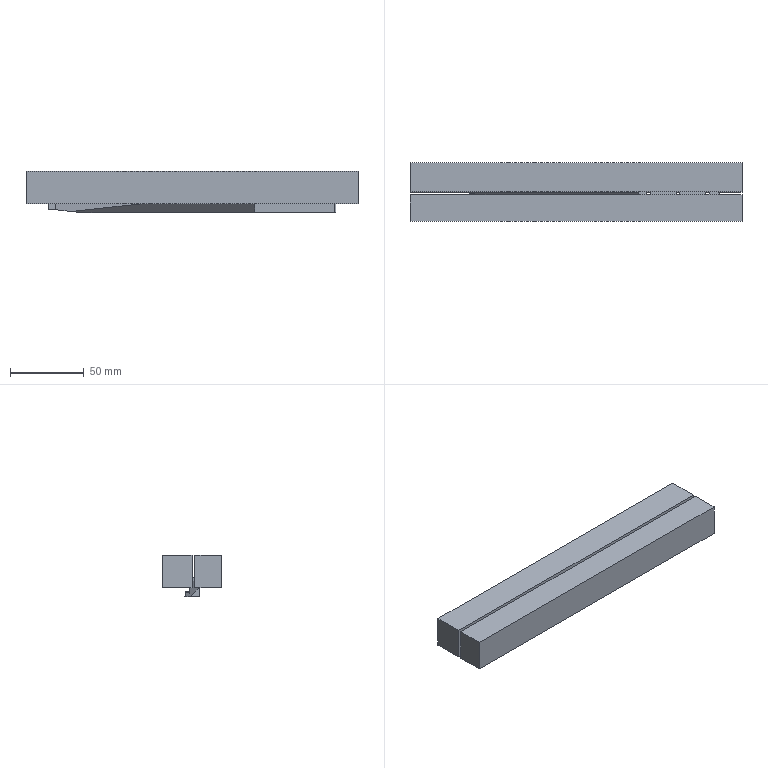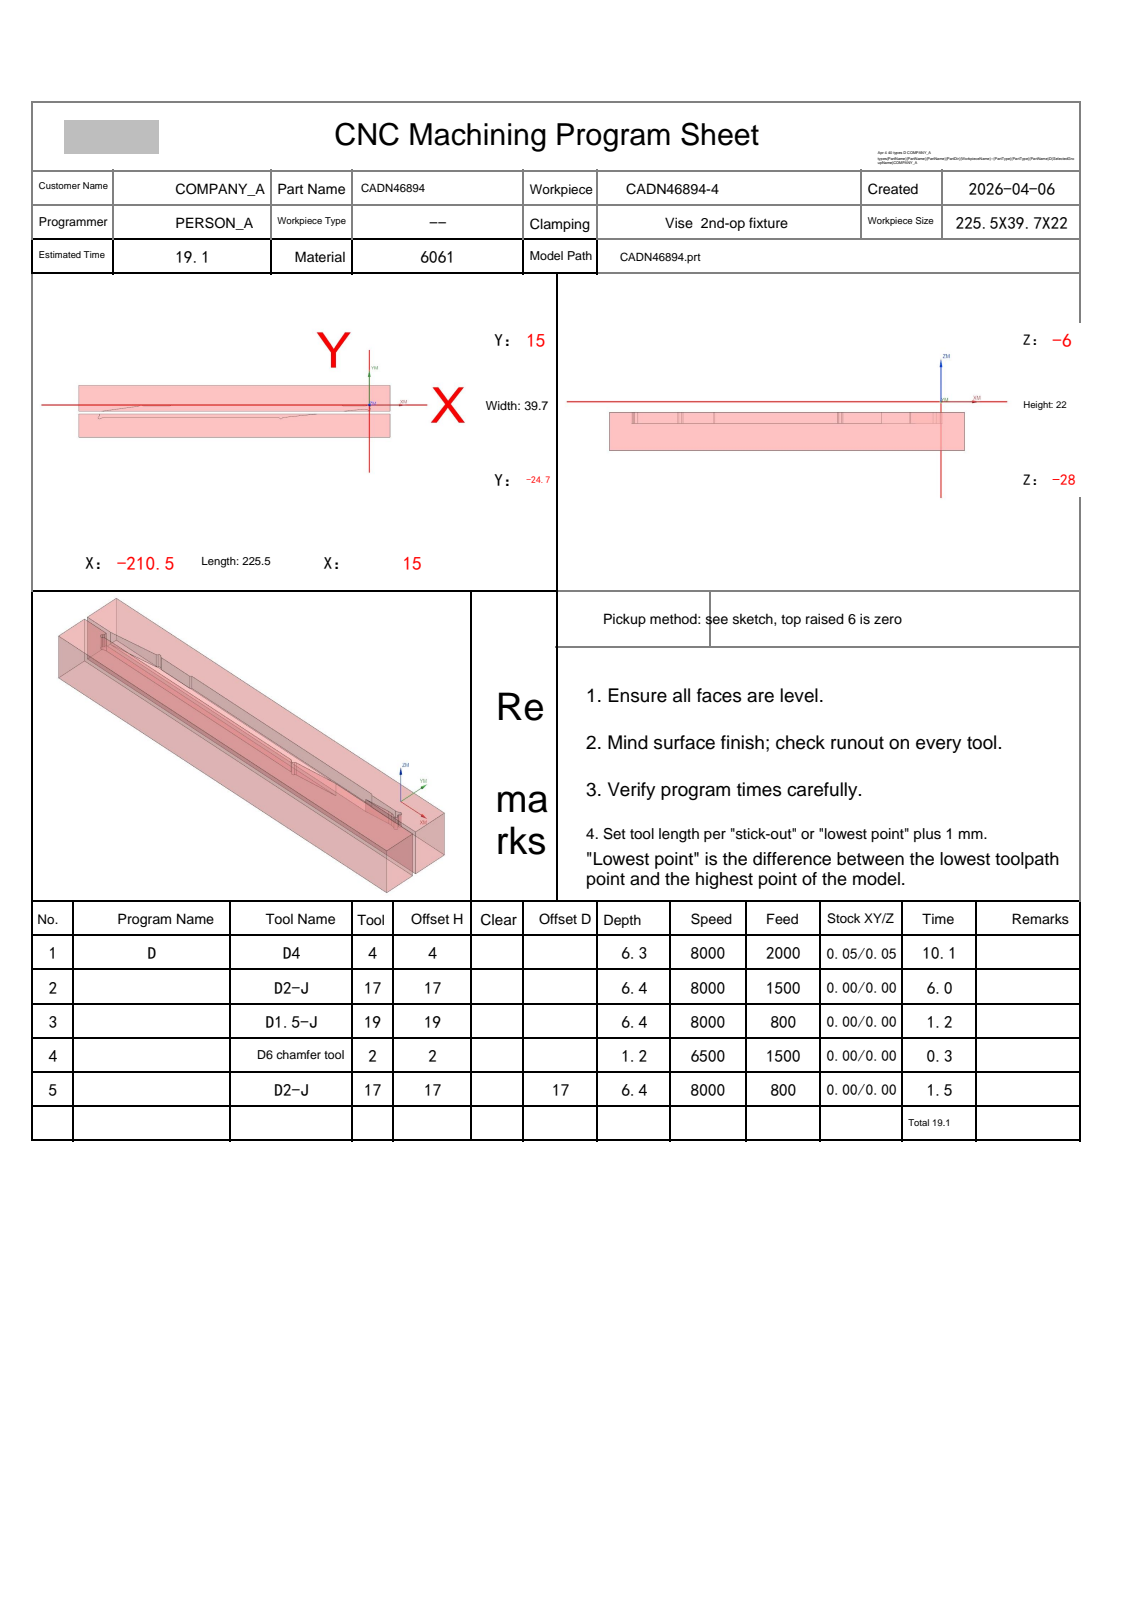NC program | NX | posted by the shop | part box 225.5 x 39.7 x 28 mm
Lines 1401 to 3483 of 3483, first 1748 of 2083 lines:
N8 T17 M06
(D2-J  D=2. R=0. H=17 ce=0.00 di=0.00)
G00 G90 G54 X-41.55 Y4.4 M03 S8000
G43 H17 Z20.
M08
Z-.2
G01 X-41.553 Y4.399 Z-.23 F800.
X-41.56 Y4.397 Z-.258
X-41.571 Y4.394 Z-.282
X-41.585 Y4.389 Z-.304
X-41.602 Y4.383 Z-.323
X-41.62 Y4.375 Z-.34
X-41.64 Y4.365 Z-.354
X-41.66 Y4.353 Z-.366
X-41.68 Y4.339 Z-.376
X-41.698 Y4.322 Z-.384
X-41.715 Y4.303 Z-.39
X-41.729 Y4.282 Z-.395
X-41.74 Y4.257 Z-.398
X-41.747 Y4.23 Z-.399
X-41.75 Y4.2 Z-.4
Y.25
X-37.801
X-37.786 Y.264 Z-.399
X-37.797 Y.305 Z-.396
X-37.831 Y.37 Z-.393
X-37.886 Y.456 Z-.388
X-38.151 Y.812 Z-.373
X-38.406 Y1.125 Z-.364
X-38.606 Y1.361 Z-.362
X-38.843 Y1.63 Z-.363
X-39.12 Y1.936 Z-.369
X-39.43 Y2.266 Z-.38
X-39.756 Y2.602 Z-.394
X-40.077 Y2.923 Z-.41
X-40.375 Y3.211 Z-.426
X-40.639 Y3.457 Z-.441
X-40.872 Y3.665 Z-.453
X-41.185 Y3.93 Z-.47
X-41.541 Y4.207 Z-.489
X-41.629 Y4.265 Z-.494
X-41.694 Y4.301 Z-.497
X-41.736 Y4.313 Z-.499
X-41.75 Y4.3 Z-.5
Y.35
X-37.801
X-37.786 Y.364 Z-.499
X-37.797 Y.405 Z-.496
X-37.831 Y.47 Z-.493
X-37.886 Y.556 Z-.488
X-38.151 Y.912 Z-.473
X-38.406 Y1.225 Z-.464
X-38.606 Y1.461 Z-.462
X-38.843 Y1.73 Z-.463
X-39.12 Y2.036 Z-.469
X-39.43 Y2.366 Z-.48
X-39.756 Y2.702 Z-.494
X-40.077 Y3.023 Z-.51
X-40.375 Y3.311 Z-.526
X-40.639 Y3.557 Z-.541
X-40.872 Y3.765 Z-.553
X-41.185 Y4.03 Z-.57
X-41.541 Y4.307 Z-.589
X-41.629 Y4.365 Z-.594
X-41.694 Y4.401 Z-.597
X-41.736 Y4.413 Z-.599
X-41.75 Y4.4 Z-.6
Y.45
X-37.801
X-37.786 Y.464 Z-.599
X-37.797 Y.504 Z-.596
X-37.831 Y.567 Z-.593
X-37.886 Y.652 Z-.588
X-38.151 Y1.002 Z-.572
X-38.406 Y1.31 Z-.564
X-38.606 Y1.541 Z-.562
X-38.843 Y1.805 Z-.563
X-39.121 Y2.105 Z-.569
X-39.43 Y2.429 Z-.58
X-39.756 Y2.758 Z-.594
X-40.077 Y3.073 Z-.61
X-40.376 Y3.355 Z-.626
X-40.64 Y3.595 Z-.641
X-40.872 Y3.799 Z-.653
X-41.185 Y4.058 Z-.67
X-41.541 Y4.329 Z-.689
X-41.629 Y4.385 Z-.694
X-41.694 Y4.42 Z-.697
X-41.736 Y4.432 Z-.699
X-41.75 Y4.418 Z-.7
Y.55
X-37.81
X-37.795 Y.564 Z-.699
X-37.806 Y.604 Z-.696
X-37.84 Y.669 Z-.693
X-37.895 Y.754 Z-.688
X-38.159 Y1.107 Z-.673
X-38.413 Y1.418 Z-.664
X-38.613 Y1.652 Z-.662
X-38.849 Y1.918 Z-.663
X-39.126 Y2.221 Z-.669
X-39.435 Y2.548 Z-.68
X-39.76 Y2.882 Z-.694
X-40.081 Y3.199 Z-.71
X-40.378 Y3.485 Z-.726
X-40.642 Y3.728 Z-.741
X-40.874 Y3.934 Z-.753
X-41.186 Y4.196 Z-.77
X-41.542 Y4.47 Z-.789
X-41.629 Y4.528 Z-.794
X-41.695 Y4.563 Z-.797
X-41.736 Y4.575 Z-.799
X-41.75 Y4.561 Z-.8
Y.65
X-37.805
X-37.79 Y.664 Z-.799
X-37.801 Y.705 Z-.796
X-37.835 Y.769 Z-.793
X-37.89 Y.856 Z-.788
X-38.155 Y1.21 Z-.773
X-38.409 Y1.524 Z-.764
X-38.609 Y1.759 Z-.762
X-38.846 Y2.027 Z-.763
X-39.123 Y2.332 Z-.769
X-39.432 Y2.661 Z-.78
X-39.758 Y2.997 Z-.794
X-40.079 Y3.317 Z-.81
X-40.377 Y3.604 Z-.826
X-40.64 Y3.849 Z-.841
X-40.873 Y4.057 Z-.853
X-41.185 Y4.321 Z-.87
X-41.542 Y4.597 Z-.889
X-41.629 Y4.655 Z-.894
X-41.695 Y4.691 Z-.897
X-41.736 Y4.703 Z-.899
X-41.75 Y4.69 Z-.9
Y.75
X-37.801
X-37.787 Y.764 Z-.899
X-37.798 Y.805 Z-.896
X-37.832 Y.87 Z-.893
X-37.887 Y.956 Z-.888
X-38.152 Y1.312 Z-.873
X-38.407 Y1.625 Z-.864
X-38.607 Y1.861 Z-.862
X-38.843 Y2.13 Z-.863
X-39.121 Y2.436 Z-.869
X-39.431 Y2.766 Z-.88
X-39.757 Y3.102 Z-.894
X-40.077 Y3.423 Z-.91
X-40.376 Y3.711 Z-.926
X-40.64 Y3.957 Z-.941
X-40.872 Y4.165 Z-.953
X-41.185 Y4.43 Z-.97
X-41.542 Y4.707 Z-.989
X-41.629 Y4.765 Z-.994
X-41.695 Y4.801 Z-.997
X-41.736 Y4.813 Z-.999
X-41.75 Y4.8 Z-1.
Y.85
X-37.8
X-37.786 Y.864 Z-.999
X-37.797 Y.904 Z-.996
X-37.831 Y.968 Z-.993
X-37.886 Y1.054 Z-.988
X-38.151 Y1.406 Z-.973
X-38.406 Y1.716 Z-.964
X-38.606 Y1.949 Z-.962
X-38.843 Y2.215 Z-.963
X-39.121 Y2.517 Z-.969
X-39.43 Y2.843 Z-.98
X-39.756 Y3.176 Z-.994
X-40.077 Y3.492 Z-1.01
X-40.375 Y3.777 Z-1.026
X-40.64 Y4.019 Z-1.041
X-40.872 Y4.225 Z-1.053
X-41.185 Y4.486 Z-1.07
X-41.541 Y4.76 Z-1.089
X-41.629 Y4.817 Z-1.094
X-41.694 Y4.852 Z-1.097
X-41.736 Y4.864 Z-1.099
X-41.75 Y4.85 Z-1.1
Y.948
X-37.801
X-37.787 Y.961 Z-1.099
X-37.798 Y1.001 Z-1.096
X-37.832 Y1.063 Z-1.093
X-37.887 Y1.147 Z-1.088
X-38.152 Y1.491 Z-1.072
X-38.407 Y1.795 Z-1.064
X-38.607 Y2.022 Z-1.062
X-38.844 Y2.282 Z-1.063
X-39.121 Y2.577 Z-1.069
X-39.431 Y2.896 Z-1.08
X-39.757 Y3.221 Z-1.094
X-40.078 Y3.53 Z-1.11
X-40.376 Y3.807 Z-1.126
X-40.64 Y4.044 Z-1.141
X-40.873 Y4.244 Z-1.153
X-41.185 Y4.498 Z-1.17
X-41.542 Y4.764 Z-1.189
X-41.629 Y4.819 Z-1.194
X-41.695 Y4.853 Z-1.197
X-41.736 Y4.864 Z-1.199
X-41.75 Y4.85 Z-1.2
Y1.05
X-37.805
X-37.79 Y1.063 Z-1.199
X-37.801 Y1.102 Z-1.196
X-37.835 Y1.163 Z-1.193
X-37.89 Y1.245 Z-1.188
X-38.155 Y1.581 Z-1.172
X-38.409 Y1.878 Z-1.164
X-38.609 Y2.1 Z-1.162
X-38.846 Y2.353 Z-1.163
X-39.123 Y2.641 Z-1.169
X-39.433 Y2.952 Z-1.18
X-39.759 Y3.268 Z-1.194
X-40.079 Y3.569 Z-1.21
X-40.377 Y3.839 Z-1.226
X-40.641 Y4.069 Z-1.241
X-40.873 Y4.264 Z-1.253
X-41.185 Y4.511 Z-1.27
X-41.542 Y4.768 Z-1.289
X-41.629 Y4.822 Z-1.294
X-41.695 Y4.854 Z-1.297
X-41.736 Y4.864 Z-1.299
X-41.75 Y4.85 Z-1.3
Y1.15
X-37.81
X-37.795 Y1.163 Z-1.299
X-37.806 Y1.201 Z-1.296
X-37.84 Y1.261 Z-1.293
X-37.895 Y1.341 Z-1.288
X-38.159 Y1.669 Z-1.272
X-38.413 Y1.958 Z-1.264
X-38.613 Y2.175 Z-1.262
X-38.849 Y2.423 Z-1.263
X-39.127 Y2.703 Z-1.269
X-39.436 Y3.006 Z-1.28
X-39.761 Y3.314 Z-1.294
X-40.081 Y3.607 Z-1.31
X-40.379 Y3.87 Z-1.326
X-40.642 Y4.094 Z-1.341
X-40.888 Y4.294 Z-1.354
X-41.248 Y4.57 Z-1.374
X-41.542 Y4.773 Z-1.389
X-41.629 Y4.824 Z-1.394
X-41.695 Y4.855 Z-1.397
X-41.736 Y4.865 Z-1.399
X-41.75 Y4.85 Z-1.4
Y1.25
X-37.817
X-37.802 Y1.263 Z-1.399
X-37.813 Y1.299 Z-1.396
X-37.847 Y1.358 Z-1.393
X-37.901 Y1.436 Z-1.388
X-38.166 Y1.757 Z-1.372
X-38.419 Y2.039 Z-1.364
X-38.619 Y2.251 Z-1.362
X-38.854 Y2.492 Z-1.363
X-39.131 Y2.765 Z-1.369
X-39.44 Y3.06 Z-1.38
X-39.765 Y3.36 Z-1.394
X-40.084 Y3.645 Z-1.41
X-40.381 Y3.901 Z-1.426
X-40.644 Y4.118 Z-1.441
X-40.89 Y4.313 Z-1.454
X-41.249 Y4.58 Z-1.474
X-41.542 Y4.777 Z-1.489
X-41.629 Y4.827 Z-1.494
X-41.695 Y4.857 Z-1.497
X-41.736 Y4.865 Z-1.499
X-41.75 Y4.85 Z-1.5
Y1.35
X-37.826
X-37.811 Y1.362 Z-1.499
X-37.822 Y1.398 Z-1.496
X-37.856 Y1.455 Z-1.493
X-37.91 Y1.532 Z-1.488
X-38.125 Y1.79 Z-1.475
X-38.415 Y2.108 Z-1.464
X-38.625 Y2.326 Z-1.462
X-38.861 Y2.561 Z-1.463
X-39.137 Y2.827 Z-1.469
X-39.445 Y3.114 Z-1.48
X-39.769 Y3.406 Z-1.494
X-40.088 Y3.683 Z-1.51
X-40.384 Y3.932 Z-1.526
X-40.647 Y4.143 Z-1.541
X-40.892 Y4.332 Z-1.554
X-41.25 Y4.591 Z-1.574
X-41.543 Y4.782 Z-1.589
X-41.63 Y4.829 Z-1.594
X-41.695 Y4.858 Z-1.597
X-41.736 Y4.865 Z-1.599
X-41.75 Y4.85 Z-1.6
Y1.45
X-37.837
X-37.822 Y1.462 Z-1.599
X-37.833 Y1.497 Z-1.596
X-37.866 Y1.553 Z-1.593
X-37.921 Y1.627 Z-1.588
X-38.135 Y1.879 Z-1.575
X-38.424 Y2.189 Z-1.564
X-38.634 Y2.402 Z-1.562
X-38.869 Y2.63 Z-1.563
X-39.144 Y2.889 Z-1.569
X-39.451 Y3.169 Z-1.58
X-39.774 Y3.452 Z-1.594
X-40.092 Y3.722 Z-1.61
X-40.388 Y3.963 Z-1.626
X-40.653 Y4.171 Z-1.641
X-40.908 Y4.361 Z-1.655
X-41.309 Y4.641 Z-1.677
X-41.543 Y4.786 Z-1.689
X-41.63 Y4.832 Z-1.694
X-41.695 Y4.859 Z-1.697
X-41.736 Y4.866 Z-1.699
X-41.75 Y4.85 Z-1.7
Y1.55
X-37.85
X-37.835 Y1.564 Z-1.699
X-37.851 Y1.605 Z-1.696
X-37.893 Y1.67 Z-1.691
X-37.96 Y1.756 Z-1.686
X-38.217 Y2.044 Z-1.671
X-38.595 Y2.428 Z-1.662
X-38.86 Y2.683 Z-1.663
X-39.142 Y2.942 Z-1.669
X-39.453 Y3.217 Z-1.68
X-39.777 Y3.496 Z-1.694
X-40.096 Y3.759 Z-1.71
X-40.392 Y3.993 Z-1.726
X-40.656 Y4.195 Z-1.741
X-40.911 Y4.38 Z-1.755
X-41.31 Y4.651 Z-1.777
X-41.544 Y4.791 Z-1.789
X-41.63 Y4.835 Z-1.794
X-41.695 Y4.86 Z-1.797
X-41.736 Y4.866 Z-1.799
X-41.75 Y4.85 Z-1.8
Y1.65
X-37.865
X-37.851 Y1.664 Z-1.799
X-37.866 Y1.704 Z-1.796
X-37.908 Y1.767 Z-1.791
X-37.975 Y1.851 Z-1.786
X-38.23 Y2.131 Z-1.771
X-38.607 Y2.505 Z-1.762
X-38.871 Y2.752 Z-1.763
X-39.152 Y3.004 Z-1.769
X-39.461 Y3.272 Z-1.78
X-39.785 Y3.542 Z-1.794
X-40.102 Y3.797 Z-1.81
X-40.397 Y4.024 Z-1.826
X-40.66 Y4.22 Z-1.841
X-40.914 Y4.399 Z-1.855
X-41.312 Y4.66 Z-1.877
X-41.544 Y4.795 Z-1.889
X-41.631 Y4.837 Z-1.894
X-41.695 Y4.861 Z-1.897
X-41.736 Y4.866 Z-1.899
X-41.75 Y4.85 Z-1.9
Y1.75
X-37.882
X-37.868 Y1.764 Z-1.899
X-37.883 Y1.802 Z-1.896
X-37.925 Y1.864 Z-1.891
X-37.991 Y1.946 Z-1.886
X-38.245 Y2.218 Z-1.871
X-38.409 Y2.382 Z-1.865
X-38.622 Y2.587 Z-1.861
X-39.177 Y3.087 Z-1.866
X-39.982 Y3.742 Z-1.903
X-40.655 Y4.237 Z-1.94
X-41.167 Y4.58 Z-1.969
X-41.505 Y4.779 Z-1.987
X-41.607 Y4.829 Z-1.993
X-41.684 Y4.859 Z-1.997
X-41.733 Y4.867 Z-1.999
X-41.75 Y4.85 Z-2.
Y1.85
X-37.902
X-37.887 Y1.863 Z-1.999
X-37.902 Y1.901 Z-1.996
X-37.943 Y1.961 Z-1.991
X-38.009 Y2.04 Z-1.986
X-38.262 Y2.305 Z-1.971
X-38.425 Y2.465 Z-1.965
X-38.682 Y2.705 Z-1.96
X-39.189 Y3.149 Z-1.966
X-39.991 Y3.783 Z-2.003
X-40.676 Y4.272 Z-2.041
X-41.237 Y4.633 Z-2.073
X-41.506 Y4.784 Z-2.087
X-41.608 Y4.833 Z-2.093
X-41.685 Y4.861 Z-2.097
X-41.733 Y4.867 Z-2.099
X-41.75 Y4.85 Z-2.1
Y1.95
X-37.923
X-37.908 Y1.963 Z-2.099
X-37.923 Y2. Z-2.096
X-37.964 Y2.058 Z-2.091
X-38.03 Y2.135 Z-2.086
X-38.281 Y2.392 Z-2.071
X-38.443 Y2.547 Z-2.065
X-38.698 Y2.78 Z-2.06
X-39.202 Y3.211 Z-2.066
X-40. Y3.824 Z-2.103
X-40.681 Y4.297 Z-2.141
X-41.239 Y4.645 Z-2.173
X-41.507 Y4.79 Z-2.187
X-41.609 Y4.836 Z-2.193
X-41.685 Y4.862 Z-2.197
X-41.733 Y4.868 Z-2.199
X-41.75 Y4.85 Z-2.2
Y2.05
X-37.947
X-37.932 Y2.062 Z-2.199
X-37.946 Y2.098 Z-2.196
X-37.987 Y2.155 Z-2.191
X-38.052 Y2.23 Z-2.186
X-38.302 Y2.48 Z-2.171
X-38.462 Y2.629 Z-2.165
X-38.716 Y2.856 Z-2.16
X-39.216 Y3.272 Z-2.166
X-40.009 Y3.866 Z-2.203
X-40.572 Y4.248 Z-2.235
X-40.866 Y4.435 Z-2.252
X-41.242 Y4.656 Z-2.273
X-41.509 Y4.795 Z-2.287
X-41.609 Y4.839 Z-2.293
X-41.685 Y4.864 Z-2.297
X-41.733 Y4.868 Z-2.299
X-41.75 Y4.85 Z-2.3
Y2.15
X-37.972
X-37.958 Y2.162 Z-2.299
X-37.972 Y2.197 Z-2.296
X-38.012 Y2.252 Z-2.291
X-38.076 Y2.324 Z-2.286
X-38.324 Y2.567 Z-2.271
X-38.484 Y2.712 Z-2.265
X-38.735 Y2.931 Z-2.26
X-39.232 Y3.334 Z-2.266
X-40.02 Y3.907 Z-2.303
X-40.58 Y4.276 Z-2.335
X-40.872 Y4.455 Z-2.352
X-41.245 Y4.667 Z-2.373
X-41.51 Y4.8 Z-2.387
X-41.61 Y4.842 Z-2.393
X-41.686 Y4.865 Z-2.397
X-41.733 Y4.868 Z-2.399
X-41.75 Y4.85 Z-2.4
Y2.25
X-38.
X-37.986 Y2.262 Z-2.399
X-37.999 Y2.295 Z-2.396
X-38.039 Y2.348 Z-2.391
X-38.103 Y2.419 Z-2.386
X-38.297 Y2.607 Z-2.374
X-38.513 Y2.8 Z-2.365
X-38.8 Y3.042 Z-2.36
X-39.25 Y3.396 Z-2.366
X-40.032 Y3.948 Z-2.403
X-40.587 Y4.303 Z-2.435
X-40.877 Y4.476 Z-2.452
X-41.248 Y4.679 Z-2.473
X-41.512 Y4.806 Z-2.487
X-41.611 Y4.845 Z-2.493
X-41.686 Y4.867 Z-2.497
X-41.733 Y4.869 Z-2.499
X-41.75 Y4.85 Z-2.5
Y2.35
X-38.031
X-38.016 Y2.361 Z-2.499
X-38.029 Y2.394 Z-2.496
X-38.069 Y2.445 Z-2.491
X-38.132 Y2.514 Z-2.486
X-38.324 Y2.696 Z-2.474
X-38.538 Y2.882 Z-2.465
X-38.823 Y3.117 Z-2.46
X-39.268 Y3.457 Z-2.466
X-39.922 Y3.91 Z-2.496
X-40.574 Y4.317 Z-2.533
X-40.896 Y4.502 Z-2.552
X-41.316 Y4.722 Z-2.576
X-41.513 Y4.811 Z-2.587
X-41.612 Y4.848 Z-2.593
X-41.687 Y4.868 Z-2.597
X-41.734 Y4.869 Z-2.599
X-41.75 Y4.85 Z-2.6
Y2.45
X-38.063
X-38.048 Y2.461 Z-2.599
X-38.061 Y2.492 Z-2.596
X-38.1 Y2.542 Z-2.591
X-38.162 Y2.608 Z-2.586
X-38.353 Y2.784 Z-2.574
X-38.565 Y2.965 Z-2.565
X-38.847 Y3.191 Z-2.56
X-39.288 Y3.519 Z-2.566
X-39.716 Y3.813 Z-2.584
X-40.158 Y4.096 Z-2.608
X-40.756 Y4.444 Z-2.644
X-41.028 Y4.588 Z-2.66
X-41.396 Y4.767 Z-2.681
X-41.515 Y4.816 Z-2.687
X-41.613 Y4.851 Z-2.693
X-41.687 Y4.869 Z-2.697
X-41.734 Y4.87 Z-2.699
X-41.75 Y4.85 Z-2.7
Y2.55
X-38.098
X-38.083 Y2.561 Z-2.699
X-38.096 Y2.591 Z-2.696
X-38.134 Y2.639 Z-2.691
X-38.196 Y2.703 Z-2.686
X-38.384 Y2.873 Z-2.674
X-38.594 Y3.047 Z-2.665
X-38.873 Y3.265 Z-2.66
X-39.31 Y3.581 Z-2.666
X-39.734 Y3.863 Z-2.684
X-40.171 Y4.134 Z-2.708
X-40.764 Y4.467 Z-2.744
X-41.034 Y4.605 Z-2.76
X-41.399 Y4.775 Z-2.781
X-41.517 Y4.822 Z-2.787
X-41.614 Y4.854 Z-2.793
X-41.687 Y4.871 Z-2.797
X-41.734 Y4.87 Z-2.799
X-41.75 Y4.85 Z-2.8
Y2.65
X-38.136
X-38.12 Y2.66 Z-2.799
X-38.133 Y2.69 Z-2.796
X-38.17 Y2.736 Z-2.791
X-38.231 Y2.798 Z-2.786
X-38.417 Y2.961 Z-2.774
X-38.625 Y3.129 Z-2.765
X-38.9 Y3.339 Z-2.76
X-39.333 Y3.642 Z-2.766
X-39.752 Y3.913 Z-2.784
X-40.186 Y4.173 Z-2.808
X-40.773 Y4.491 Z-2.844
X-41.04 Y4.622 Z-2.86
X-41.402 Y4.783 Z-2.881
X-41.519 Y4.827 Z-2.887
X-41.615 Y4.857 Z-2.893
X-41.688 Y4.872 Z-2.897
X-41.734 Y4.87 Z-2.899
X-41.75 Y4.85 Z-2.9
Y2.75
X-38.176
X-38.16 Y2.76 Z-2.899
X-38.172 Y2.788 Z-2.896
X-38.209 Y2.833 Z-2.891
X-38.269 Y2.892 Z-2.886
X-38.405 Y3.011 Z-2.876
X-38.647 Y3.204 Z-2.865
X-38.93 Y3.413 Z-2.86
X-39.358 Y3.704 Z-2.866
X-39.772 Y3.963 Z-2.884
X-40.201 Y4.211 Z-2.908
X-40.783 Y4.514 Z-2.944
X-41.047 Y4.639 Z-2.96
X-41.405 Y4.791 Z-2.981
X-41.521 Y4.832 Z-2.987
X-41.616 Y4.86 Z-2.993
X-41.689 Y4.874 Z-2.997
X-41.734 Y4.871 Z-2.999
X-41.75 Y4.85 Z-3.
Y2.85
X-38.218
X-38.202 Y2.862 Z-2.999
X-38.22 Y2.895 Z-2.995
X-38.267 Y2.947 Z-2.989
X-38.341 Y3.016 Z-2.983
X-38.562 Y3.195 Z-2.97
X-38.721 Y3.315 Z-2.964
X-39. Y3.514 Z-2.959
X-39.384 Y3.766 Z-2.966
X-39.793 Y4.013 Z-2.984
X-40.217 Y4.25 Z-3.008
X-40.793 Y4.537 Z-3.044
X-41.054 Y4.656 Z-3.06
X-41.409 Y4.799 Z-3.081
X-41.523 Y4.838 Z-3.087
X-41.618 Y4.863 Z-3.093
X-41.689 Y4.875 Z-3.097
X-41.734 Y4.871 Z-3.099
X-41.75 Y4.85 Z-3.1
Y2.95
X-38.263
X-38.247 Y2.961 Z-3.099
X-38.264 Y2.993 Z-3.095
X-38.31 Y3.044 Z-3.089
X-38.383 Y3.11 Z-3.083
X-38.601 Y3.282 Z-3.07
X-38.757 Y3.396 Z-3.064
X-39.032 Y3.587 Z-3.059
X-39.411 Y3.827 Z-3.066
X-39.816 Y4.063 Z-3.084
X-40.234 Y4.288 Z-3.108
X-40.803 Y4.561 Z-3.144
X-41.062 Y4.672 Z-3.16
X-41.412 Y4.808 Z-3.181
X-41.526 Y4.843 Z-3.187
X-41.619 Y4.867 Z-3.193
X-41.69 Y4.876 Z-3.197
X-41.734 Y4.871 Z-3.199
X-41.75 Y4.85 Z-3.2
Y3.05
X-38.311
X-38.294 Y3.061 Z-3.199
X-38.311 Y3.092 Z-3.195
X-38.356 Y3.14 Z-3.189
X-38.428 Y3.203 Z-3.183
X-38.588 Y3.328 Z-3.173
X-38.796 Y3.478 Z-3.164
X-39.067 Y3.659 Z-3.159
X-39.441 Y3.889 Z-3.166
X-39.84 Y4.113 Z-3.184
X-40.253 Y4.326 Z-3.208
X-40.777 Y4.569 Z-3.241
X-41.024 Y4.671 Z-3.257
X-41.346 Y4.793 Z-3.276
X-41.481 Y4.835 Z-3.284
X-41.592 Y4.864 Z-3.291
X-41.677 Y4.877 Z-3.296
X-41.731 Y4.873 Z-3.299
X-41.75 Y4.85 Z-3.3
Y3.15
X-38.361
X-38.345 Y3.16 Z-3.299
X-38.36 Y3.19 Z-3.295
X-38.405 Y3.236 Z-3.289
X-38.475 Y3.297 Z-3.283
X-38.632 Y3.416 Z-3.273
X-38.837 Y3.559 Z-3.264
X-39.104 Y3.732 Z-3.259
X-39.472 Y3.95 Z-3.266
X-39.865 Y4.163 Z-3.284
X-40.272 Y4.365 Z-3.308
X-40.79 Y4.593 Z-3.341
X-41.033 Y4.689 Z-3.357
X-41.351 Y4.803 Z-3.376
X-41.484 Y4.842 Z-3.384
X-41.594 Y4.868 Z-3.391
X-41.678 Y4.879 Z-3.396
X-41.731 Y4.874 Z-3.399
X-41.75 Y4.85 Z-3.4
Y3.25
X-38.414
X-38.398 Y3.26 Z-3.399
X-38.413 Y3.288 Z-3.395
X-38.456 Y3.332 Z-3.389
X-38.525 Y3.39 Z-3.383
X-38.679 Y3.504 Z-3.373
X-38.88 Y3.64 Z-3.364
X-39.143 Y3.805 Z-3.359
X-39.505 Y4.012 Z-3.366
X-39.891 Y4.213 Z-3.384
X-40.292 Y4.403 Z-3.408
X-40.803 Y4.617 Z-3.441
X-41.043 Y4.707 Z-3.457
X-41.357 Y4.812 Z-3.476
X-41.487 Y4.848 Z-3.484
X-41.596 Y4.872 Z-3.491
X-41.679 Y4.881 Z-3.496
X-41.732 Y4.874 Z-3.499
X-41.75 Y4.85 Z-3.5
Y3.35
X-38.47
X-38.454 Y3.359 Z-3.499
X-38.468 Y3.386 Z-3.495
X-38.51 Y3.429 Z-3.489
X-38.577 Y3.484 Z-3.483
X-38.667 Y3.55 Z-3.476
X-38.913 Y3.713 Z-3.465
X-39.184 Y3.878 Z-3.459
X-39.539 Y4.074 Z-3.466
X-39.92 Y4.263 Z-3.484
X-40.314 Y4.441 Z-3.508
X-40.816 Y4.641 Z-3.541
X-41.053 Y4.725 Z-3.557
X-41.362 Y4.822 Z-3.576
X-41.491 Y4.855 Z-3.584
X-41.598 Y4.875 Z-3.591
X-41.68 Y4.882 Z-3.596
X-41.732 Y4.875 Z-3.599
X-41.75 Y4.85 Z-3.6
Y3.45
X-38.53
X-38.513 Y3.459 Z-3.599
X-38.526 Y3.485 Z-3.595
X-38.567 Y3.525 Z-3.589
X-38.633 Y3.577 Z-3.583
X-38.72 Y3.64 Z-3.576
X-38.961 Y3.795 Z-3.565
X-39.227 Y3.951 Z-3.559
X-39.576 Y4.135 Z-3.566
X-39.949 Y4.313 Z-3.584
X-40.337 Y4.48 Z-3.608
X-40.831 Y4.666 Z-3.641
X-41.064 Y4.743 Z-3.657
X-41.368 Y4.832 Z-3.676
X-41.495 Y4.861 Z-3.684
X-41.6 Y4.879 Z-3.691
X-41.681 Y4.884 Z-3.696
X-41.732 Y4.875 Z-3.699
X-41.75 Y4.85 Z-3.7
Y3.55
X-38.592
X-38.575 Y3.559 Z-3.699
X-38.588 Y3.583 Z-3.695
X-38.627 Y3.621 Z-3.689
X-38.691 Y3.671 Z-3.683
X-38.777 Y3.73 Z-3.676
X-39.012 Y3.877 Z-3.665
X-39.272 Y4.024 Z-3.659
X-39.614 Y4.197 Z-3.666
X-39.98 Y4.363 Z-3.684
X-40.361 Y4.518 Z-3.708
X-40.846 Y4.69 Z-3.742
X-41.075 Y4.761 Z-3.757
X-41.374 Y4.842 Z-3.776
X-41.499 Y4.868 Z-3.784
X-41.603 Y4.883 Z-3.791
X-41.682 Y4.886 Z-3.796
X-41.732 Y4.875 Z-3.799
X-41.75 Y4.85 Z-3.8
Y3.65
X-38.658
X-38.64 Y3.658 Z-3.799
X-38.652 Y3.681 Z-3.795
X-38.691 Y3.717 Z-3.789
X-38.753 Y3.764 Z-3.783
X-38.836 Y3.82 Z-3.776
X-39.066 Y3.959 Z-3.765
X-39.32 Y4.097 Z-3.759
X-39.655 Y4.259 Z-3.766
X-40.013 Y4.413 Z-3.784
X-40.386 Y4.556 Z-3.808
X-40.862 Y4.714 Z-3.842
X-41.087 Y4.779 Z-3.857
X-41.38 Y4.851 Z-3.876
X-41.503 Y4.874 Z-3.884
X-41.605 Y4.887 Z-3.891
X-41.683 Y4.888 Z-3.896
X-41.733 Y4.876 Z-3.899
X-41.75 Y4.85 Z-3.9
Y3.75
X-38.727
X-38.709 Y3.76 Z-3.898
X-38.727 Y3.787 Z-3.894
X-38.777 Y3.829 Z-3.887
X-38.856 Y3.883 Z-3.88
X-38.958 Y3.947 Z-3.872
X-39.157 Y4.059 Z-3.863
X-39.371 Y4.17 Z-3.859
X-39.698 Y4.32 Z-3.866
X-40.048 Y4.463 Z-3.884
X-40.412 Y4.595 Z-3.908
X-40.83 Y4.725 Z-3.938
X-41.099 Y4.797 Z-3.957
X-41.387 Y4.861 Z-3.976
X-41.508 Y4.881 Z-3.984
X-41.608 Y4.89 Z-3.991
X-41.684 Y4.889 Z-3.996
X-41.733 Y4.876 Z-3.999
X-41.75 Y4.85 Z-4.
Y3.85
X-38.801
X-38.782 Y3.859 Z-3.998
X-38.799 Y3.885 Z-3.994
X-38.847 Y3.924 Z-3.987
X-38.923 Y3.975 Z-3.98
X-39.023 Y4.035 Z-3.972
X-39.216 Y4.14 Z-3.963
X-39.424 Y4.243 Z-3.959
X-39.743 Y4.382 Z-3.966
X-40.085 Y4.513 Z-3.984
X-40.44 Y4.633 Z-4.008
X-40.848 Y4.751 Z-4.038
X-41.112 Y4.815 Z-4.057
X-41.394 Y4.871 Z-4.076
X-41.512 Y4.887 Z-4.084
X-41.611 Y4.894 Z-4.091
X-41.686 Y4.891 Z-4.096
X-41.733 Y4.877 Z-4.099
X-41.75 Y4.85 Z-4.1
Y3.95
X-38.877
X-38.859 Y3.959 Z-4.098
X-38.874 Y3.983 Z-4.094
X-38.92 Y4.02 Z-4.087
X-38.994 Y4.067 Z-4.08
X-39.09 Y4.123 Z-4.072
X-39.278 Y4.22 Z-4.063
X-39.48 Y4.316 Z-4.059
X-39.79 Y4.444 Z-4.066
X-40.123 Y4.563 Z-4.084
X-40.47 Y4.671 Z-4.108
X-40.868 Y4.776 Z-4.138
X-41.126 Y4.833 Z-4.157
X-41.402 Y4.881 Z-4.176
X-41.517 Y4.894 Z-4.184
X-41.614 Y4.898 Z-4.191
X-41.687 Y4.893 Z-4.196
X-41.734 Y4.877 Z-4.199
X-41.75 Y4.85 Z-4.2
Y4.05
X-38.959
X-38.939 Y4.058 Z-4.198
X-38.953 Y4.08 Z-4.194
X-38.998 Y4.115 Z-4.187
X-39.068 Y4.159 Z-4.18
X-39.162 Y4.211 Z-4.172
X-39.274 Y4.268 Z-4.166
X-39.401 Y4.328 Z-4.161
X-39.54 Y4.389 Z-4.159
X-39.84 Y4.505 Z-4.166
X-40.164 Y4.613 Z-4.184
X-40.501 Y4.71 Z-4.208
X-40.899 Y4.804 Z-4.239
X-41.092 Y4.842 Z-4.253
X-41.332 Y4.881 Z-4.271
X-41.468 Y4.896 Z-4.281
X-41.584 Y4.902 Z-4.289
X-41.673 Y4.897 Z-4.295
X-41.73 Y4.88 Z-4.299
X-41.75 Y4.85 Z-4.3
Y4.15
X-39.044
X-39.024 Y4.157 Z-4.298
X-39.037 Y4.178 Z-4.294
X-39.079 Y4.21 Z-4.287
X-39.147 Y4.251 Z-4.28
X-39.237 Y4.299 Z-4.272
X-39.345 Y4.351 Z-4.266
X-39.468 Y4.406 Z-4.261
X-39.602 Y4.462 Z-4.259
X-39.893 Y4.567 Z-4.266
X-40.206 Y4.663 Z-4.284
X-40.534 Y4.748 Z-4.308
X-40.92 Y4.829 Z-4.339
X-41.108 Y4.861 Z-4.353
X-41.342 Y4.893 Z-4.371
X-41.475 Y4.904 Z-4.381
X-41.588 Y4.907 Z-4.389
X-41.675 Y4.899 Z-4.395
X-41.73 Y4.881 Z-4.399
X-41.75 Y4.85 Z-4.4
Y4.25
X-39.134
X-39.114 Y4.257 Z-4.398
X-39.125 Y4.276 Z-4.394
X-39.165 Y4.305 Z-4.387
X-39.23 Y4.343 Z-4.38
X-39.316 Y4.387 Z-4.372
X-39.42 Y4.435 Z-4.366
X-39.538 Y4.484 Z-4.361
X-39.668 Y4.534 Z-4.359
X-39.949 Y4.629 Z-4.366
X-40.252 Y4.713 Z-4.384
X-40.569 Y4.786 Z-4.408
X-40.943 Y4.855 Z-4.439
X-41.126 Y4.881 Z-4.453
X-41.353 Y4.905 Z-4.471
X-41.483 Y4.912 Z-4.481
X-41.592 Z-4.489
X-41.677 Y4.902 Z-4.495
X-41.731 Y4.881 Z-4.499
X-41.75 Y4.85 Z-4.5
Y4.35
X-39.23
X-39.209 Y4.356 Z-4.498
X-39.219 Y4.374 Z-4.494
X-39.256 Y4.401 Z-4.487
X-39.318 Y4.435 Z-4.48
X-39.4 Y4.475 Z-4.472
X-39.499 Y4.518 Z-4.466
X-39.613 Y4.563 Z-4.461
X-39.737 Y4.607 Z-4.459
X-40.008 Y4.69 Z-4.466
X-40.299 Y4.763 Z-4.484
X-40.605 Y4.825 Z-4.508
X-40.968 Y4.88 Z-4.539
X-41.144 Y4.9 Z-4.553
X-41.364 Y4.917 Z-4.571
X-41.49 Y4.921 Z-4.581
X-41.597 Y4.916 Z-4.589
X-41.679 Y4.904 Z-4.595
X-41.731 Y4.882 Z-4.599
X-41.75 Y4.85 Z-4.6
Y4.45
X-39.331
X-39.309 Y4.456 Z-4.598
X-39.317 Y4.472 Z-4.594
X-39.352 Y4.496 Z-4.587
X-39.41 Y4.527 Z-4.58
X-39.488 Y4.562 Z-4.572
X-39.583 Y4.601 Z-4.566
X-39.692 Y4.641 Z-4.561
X-39.811 Y4.68 Z-4.559
X-40.07 Y4.752 Z-4.566
X-40.35 Y4.813 Z-4.584
X-40.644 Y4.863 Z-4.608
X-40.994 Y4.905 Z-4.639
X-41.164 Y4.919 Z-4.653
X-41.377 Y4.929 Z-4.671
X-41.498 Z-4.681
X-41.601 Y4.921 Z-4.689
X-41.681 Y4.906 Z-4.695
X-41.732 Y4.883 Z-4.699
X-41.75 Y4.85 Z-4.7
Y4.55
X-39.437
X-39.415 Y4.557 Z-4.698
X-39.429 Y4.575 Z-4.692
X-39.475 Y4.602 Z-4.684
X-39.549 Y4.636 Z-4.675
X-39.645 Y4.675 Z-4.667
X-39.76 Y4.714 Z-4.662
X-39.889 Y4.753 Z-4.659
X-40.136 Y4.814 Z-4.666
X-40.403 Y4.863 Z-4.684
X-40.685 Y4.901 Z-4.708
X-41.021 Y4.931 Z-4.739
X-41.185 Y4.939 Z-4.753
X-41.389 Y4.942 Z-4.771
X-41.507 Y4.937 Z-4.781
X-41.606 Y4.926 Z-4.789
X-41.683 Y4.908 Z-4.795
X-41.733 Y4.883 Z-4.799
X-41.75 Y4.85 Z-4.8
Y4.65
X-39.551
X-39.549 Y4.653 Z-4.799
X-39.582 Y4.66 Z-4.795
X-39.825 Y4.697 Z-4.782
X-40.115 Y4.73 Z-4.774
X-40.469 Y4.757 Z-4.777
X-40.837 Y4.773 Z-4.793
X-41.191 Y4.776 Z-4.82
X-41.481 Y4.768 Z-4.853
X-41.724 Y4.755 Z-4.89
X-41.757 Y4.751 Z-4.897
X-41.755 Y4.75 Z-4.9
X-39.672
X-39.668 Y4.753 Z-4.899
X-39.699 Y4.76 Z-4.895
X-39.928 Y4.797 Z-4.882
X-40.201 Y4.83 Z-4.874
X-40.536 Y4.857 Z-4.877
X-40.885 Y4.873 Z-4.893
X-41.22 Y4.876 Z-4.92
X-41.494 Y4.868 Z-4.953
X-41.723 Y4.855 Z-4.99
X-41.753 Y4.851 Z-4.997
X-41.75 Y4.85 Z-5.
X-39.801
X-39.796 Y4.853 Z-4.999
X-39.824 Y4.86 Z-4.995
X-39.973 Y4.887 Z-4.985
X-40.086 Y4.904 Z-4.98
X-40.297 Y4.93 Z-4.974
X-40.613 Y4.957 Z-4.977
X-40.942 Y4.973 Z-4.993
X-41.259 Y4.976 Z-5.02
X-41.469 Y4.97 Z-5.046
X-41.583 Y4.965 Z-5.063
X-41.731 Y4.955 Z-5.09
X-41.759 Y4.951 Z-5.097
X-41.755 Y4.95 Z-5.1
X-39.939
X-39.933 Y4.952 Z-5.099
X-39.95 Y4.958 Z-5.096
X-39.988 Y4.967 Z-5.093
X-40.18 Y5. Z-5.081
X-40.401 Y5.03 Z-5.074
X-40.699 Y5.057 Z-5.077
X-41.01 Y5.073 Z-5.093
X-41.308 Y5.076 Z-5.12
X-41.528 Y5.069 Z-5.15
X-41.721 Y5.057 Z-5.183
X-41.759 Y5.054 Z-5.192
X-41.776 Y5.051 Z-5.198
X-41.77 Y5.05 Z-5.2
X-40.088
X-40.081 Y5.052 Z-5.199
X-40.096 Y5.058 Z-5.196
X-40.131 Y5.067 Z-5.193
X-40.258 Y5.092 Z-5.183
X-40.351 Y5.107 Z-5.179
X-40.517 Y5.13 Z-5.174
X-40.724 Y5.151 Z-5.175
X-40.942 Y5.166 Z-5.184
X-41.159 Y5.175 Z-5.199
X-41.367 Y5.176 Z-5.22
X-41.533 Y5.171 Z-5.243
X-41.625 Y5.167 Z-5.258
X-41.752 Y5.157 Z-5.283
X-41.787 Y5.154 Z-5.292
X-41.803 Y5.151 Z-5.298
X-41.796 Y5.15 Z-5.3
X-40.249
X-40.242 Y5.152 Z-5.299
X-40.255 Y5.158 Z-5.296
X-40.287 Y5.167 Z-5.293
X-40.404 Y5.192 Z-5.283
X-40.49 Y5.207 Z-5.279
X-40.645 Y5.23 Z-5.274
X-40.838 Y5.251 Z-5.275
X-41.041 Y5.266 Z-5.284
X-41.244 Y5.275 Z-5.299
X-41.438 Y5.276 Z-5.32
X-41.592 Y5.271 Z-5.343
X-41.678 Y5.267 Z-5.358
X-41.796 Y5.257 Z-5.383
X-41.828 Y5.254 Z-5.392
X-41.841 Y5.251 Z-5.398
X-41.833 Y5.25 Z-5.4
X-40.426
X-40.417 Y5.252 Z-5.399
X-40.429 Y5.258 Z-5.396
X-40.458 Y5.267 Z-5.393
X-40.502 Y5.278 Z-5.388
X-40.637 Y5.305 Z-5.379
X-40.787 Y5.33 Z-5.374
X-40.967 Y5.351 Z-5.375
X-41.155 Y5.366 Z-5.384
X-41.343 Y5.375 Z-5.399
X-41.522 Y5.376 Z-5.42
X-41.673 Y5.371 Z-5.445
X-41.808 Y5.362 Z-5.472
X-41.852 Y5.357 Z-5.483
X-41.881 Y5.354 Z-5.492
X-41.892 Y5.351 Z-5.498
X-41.884 Y5.35 Z-5.5
X-40.621
X-40.612 Y5.352 Z-5.499
X-40.621 Y5.358 Z-5.496
X-40.647 Y5.367 Z-5.493
X-40.687 Y5.378 Z-5.488
X-40.774 Y5.398 Z-5.481
X-40.839 Y5.411 Z-5.478
X-40.948 Y5.43 Z-5.474
X-41.112 Y5.451 Z-5.475
X-41.286 Y5.466 Z-5.484
X-41.459 Y5.475 Z-5.499
X-41.623 Y5.476 Z-5.52
X-41.732 Y5.472 Z-5.539
X-41.797 Y5.469 Z-5.552
X-41.884 Y5.462 Z-5.572
X-41.924 Y5.457 Z-5.583
X-41.95 Y5.454 Z-5.592
X-41.959 Y5.451 Z-5.598
X-41.95 Y5.45 Z-5.6
X-40.841
X-40.831 Y5.452 Z-5.599
X-40.838 Y5.458 Z-5.596
X-40.86 Y5.467 Z-5.593
X-40.896 Y5.478 Z-5.588
X-40.942 Y5.491 Z-5.584
X-40.998 Y5.504 Z-5.579
X-41.062 Y5.517 Z-5.576
X-41.131 Y5.53 Z-5.574
X-41.281 Y5.551 Z-5.575
X-41.438 Y5.566 Z-5.584
X-41.596 Y5.575 Z-5.599
X-41.746 Y5.576 Z-5.62
X-41.815 Y5.574 Z-5.633
X-41.878 Y5.571 Z-5.646
X-41.935 Y5.566 Z-5.659
X-41.981 Y5.562 Z-5.672
X-42.016 Y5.557 Z-5.683
X-42.038 Y5.554 Z-5.692
X-42.046 Y5.551 Z-5.698
X-42.036 Y5.55 Z-5.7
X-41.095
X-41.084 Y5.552 Z-5.699
X-41.089 Y5.558 Z-5.696
X-41.108 Y5.567 Z-5.693
X-41.138 Y5.578 Z-5.688
X-41.179 Y5.591 Z-5.684
X-41.229 Y5.604 Z-5.679
X-41.285 Y5.617 Z-5.676
X-41.347 Y5.63 Z-5.674
X-41.481 Y5.651 Z-5.675
X-41.622 Y5.666 Z-5.684
X-41.764 Y5.675 Z-5.699
X-41.898 Y5.676 Z-5.72
X-41.959 Y5.674 Z-5.733
X-42.016 Y5.671 Z-5.746
X-42.066 Y5.666 Z-5.759
X-42.106 Y5.662 Z-5.772
X-42.137 Y5.657 Z-5.783
X-42.156 Y5.654 Z-5.792
X-42.161 Y5.651 Z-5.798
X-42.15 Y5.65 Z-5.8
X-41.401
X-41.375 Y5.653 Z-5.798
X-41.364 Y5.661 Z-5.792
X-41.366 Y5.673 Z-5.784
X-41.38 Y5.689 Z-5.774
X-41.404 Y5.707 Z-5.763
X-41.438 Y5.726 Z-5.751
X-41.48 Y5.746 Z-5.739
X-41.528 Y5.765 Z-5.729
X-41.581 Y5.783 Z-5.721
X-41.687 Y5.809 Z-5.713
X-41.8 Y5.827 Z-5.714
X-41.915 Y5.836 Z-5.723
X-42.028 Y5.837 Z-5.741
X-42.133 Y5.829 Z-5.767
X-42.187 Y5.821 Z-5.785
X-42.235 Y5.811 Z-5.804
X-42.276 Y5.799 Z-5.824
X-42.31 Y5.787 Z-5.843
X-42.335 Y5.776 Z-5.861
X-42.349 Y5.766 Z-5.877
X-42.351 Y5.758 Z-5.889
X-42.34 Y5.752 Z-5.897
X-42.314 Y5.75 Z-5.9
X-41.806
X-41.773 Y5.752 Z-5.897
X-41.744 Y5.758 Z-5.889
X-41.718 Y5.767 Z-5.877
X-41.696 Y5.778 Z-5.86
X-41.676 Y5.791 Z-5.84
X-41.66 Y5.806 Z-5.816
X-41.646 Y5.821 Z-5.789
X-41.634 Y5.836 Z-5.76
X-41.624 Y5.85 Z-5.729
X-41.617 Y5.863 Z-5.696
X-41.612 Y5.875 Z-5.662
X-41.608 Y5.884 Z-5.628
X-41.606 Y5.889 Z-5.593
Y5.891 Z-5.559
G00 Z20.
G91 G28 Z0.0
M05
M09
G91 G28 Z0.0
M01
N9 T18 M06
(D4R0.5  D=4. R=0.5 H=18 ce=0.00 di=0.00)
G00 G90 G54 X78.892 Y-4.82 M03 S6000
G43 H18 Z20.
M08
Z2.989
G01 Z-.103 F3500.
X76.902 Y-4.627 Z-.025
X76.067 Y-4.547 Z.007
X75.798 Y-4.521 Z.015
Y-4.421
X76.067 Y-4.447 Z.008
X77.995 Y-4.633 Z-.068
X79.087 Y-4.639 Z-.111
X76.067 Y-4.347 Z.008
X75.798 Y-4.321 Z.015
Y-4.221
X76.067 Y-4.247 Z.008
X80.165 Y-4.643 Z-.153
X81.229 Y-4.645 Z-.195
X76.067 Y-4.147 Z.008
X75.798 Y-4.121 Z.015
Y-4.021
X76.067 Y-4.047 Z.008
X82.286 Y-4.648 Z-.236
X83.327 Z-.277
X76.067 Y-3.947 Z.008
X75.798 Y-3.921 Z.015
Y-3.821
X76.067 Y-3.847 Z.008
X84.367 Y-4.649 Z-.317
X85.407 Z-.358
X76.067 Y-3.747 Z.008
X75.798 Y-3.721 Z.015
Y-3.621
X76.061 Y-3.646 Z.008
X86.447 Y-4.65 Z-.399
X87.485 Z-.439
X76.067 Y-3.547 Z.008
X75.798 Y-3.521 Z.015
Y-3.421
X76.067 Y-3.447 Z.008
X88.515 Y-4.649 Z-.48
X89.546 Z-.52
X76.067 Y-3.347 Z.008
X75.798 Y-3.321 Z.015
Y-3.221
X76.061 Y-3.246 Z.008
X90.577 Y-4.648 Z-.56
X91.607 Z-.601
X76.067 Y-3.147 Z.008
X75.798 Y-3.121 Z.015
Y-3.021
X76.067 Y-3.047 Z.008
X92.638 Y-4.648 Z-.641
X93.645 Y-4.645 Z-.68
X76.067 Y-2.947 Z.008
X75.798 Y-2.921 Z.015
Y-2.821
X76.067 Y-2.847 Z.008
X94.65 Y-4.642 Z-.72
X95.635 Y-4.637 Z-.758
X76.067 Y-2.747 Z.008
X75.798 Y-2.721 Z.015
Y-2.621
X76.067 Y-2.647 Z.008
X96.605 Y-4.631 Z-.796
X97.543 Y-4.621 Z-.833
X76.067 Y-2.547 Z.008
X75.798 Y-2.521 Z.015
Y-2.421
X76.067 Y-2.447 Z.008
X98.479 Y-4.612 Z-.87
X98.667 Y-4.609 Z-.877
X98.934 Y-4.601 Z-.888
X98.981 Y-4.591 Z-.889
X99.043 Y-4.567 Z-.892
X76.067 Y-2.347 Z.008
X75.798 Y-2.321 Z.015
X75.799 Y-2.221
X76.067 Y-2.247 Z.008
X99.24 Y-4.485 Z-.899
X99.332 Y-4.446 Z-.903
X99.358 Y-4.426 Z-.904
X99.381 Y-4.4 Z-.905
X76.067 Y-2.147 Z.008
X75.799 Y-2.121 Z.015
Y-2.021
X76.067 Y-2.047 Z.008
X99.46 Y-4.307 Z-.908
X99.529 Y-4.225 Z-.911
X99.535 Y-4.214
X76.067 Y-1.947 Z.008
X75.799 Y-1.921 Z.015
Y-1.821
X76.067 Y-1.847 Z.008
X99.597 Y-4.12 Z-.913
X99.659 Y-4.026 Z-.916
X76.067 Y-1.747 Z.008
X75.799 Y-1.721 Z.015
Y-1.621
X76.067 Y-1.647 Z.008
X99.686 Y-3.929 Z-.917
X99.699 Y-3.83 Z-.918
X76.067 Y-1.547 Z.008
X75.799 Y-1.521 Z.015
Y-1.421
X76.067 Y-1.447 Z.008
X99.712 Y-3.731 Z-.918
X99.717 Y-3.699
X99.719 Y-3.632
X76.067 Y-1.347 Z.008
X75.799 Y-1.321 Z.015
Y-1.221
X76.067 Y-1.247 Z.008
X99.722 Y-3.532 Z-.919
X99.725 Y-3.432
X76.067 Y-1.147 Z.008
X75.799 Y-1.121 Z.015
Y-1.021
X76.067 Y-1.047 Z.008
X99.728 Y-3.333 Z-.919
Y-3.233
X76.067 Y-.947 Z.008
X75.799 Y-.921 Z.015
Y-.821
X76.067 Y-.847 Z.008
X99.728 Y-3.133 Z-.919
Y-3.033
X76.067 Y-.747 Z.007
X75.799 Y-.721 Z.015
X75.804 Y-.703
X75.822 Y-.697 Z.014
X76.067 Y-.686 Z.007
X76.342 Y-.673 Z-.003
X99.728 Y-2.932 Z-.919
X99.727 Y-2.832
X77.05 Y-.641 Z-.031
X77.762 Y-.609 Z-.059
X99.727 Y-2.731 Z-.919
Y-2.631
X78.476 Y-.578 Z-.087
X79.19 Y-.546 Z-.115
X99.727 Y-2.53 Z-.919
X99.726 Y-2.43
X79.917 Y-.516 Z-.143
X80.649 Y-.486 Z-.172
X99.726 Y-2.329 Z-.919
Y-2.229
X81.385 Y-.457 Z-.201
X82.138 Y-.429 Z-.23
X99.726 Y-2.128 Z-.919
X99.718 Y-2.027 Z-.918
X82.89 Y-.401 Z-.26
X83.657 Y-.375 Z-.29
X99.71 Y-1.926 Z-.918
X99.688 Y-1.823 Z-.917
X84.433 Y-.35 Z-.32
X84.97 Y-.333 Z-.341
X85.236 Y-.327 Z-.351
X99.666 Y-1.721 Z-.916
X99.644 Y-1.618
X86.063 Y-.306 Z-.384
X86.784 Y-.288 Z-.412
X87.179 Y-.315 Z-.428
X92.72 Y-.85 Z-.644
X94.308 Y-1.002 Z-.706
X99.561 Y-1.51 Z-.912
X99.468 Y-1.4 Z-.908
X95.659 Y-1.032 Z-.759
X96.957 Y-1.057 Z-.81
X99.34 Y-1.287 Z-.903
X99.171 Y-1.171 Z-.897
X98.244 Y-1.081 Z-.86
X96.255 Y-.889 Z-.783
Z2.342
G00 Z20.
G00 G90 X-43.732 Y7.072 M03 S6000
Z20.
Z2.689
G01 Z-6.515 F3500.
X-41.732
X-38.56
X-36.781 Y7.064 Z-6.507
X-34.784 Y7.06 Z-6.503
X-31.554 Y7.058 Z-6.501
X27.509 Y7.054 Z-6.498
X29.904 Y7.049 Z-6.492
X31.566 Y7.042 Z-6.486
X33.446 Y7.029 Z-6.473
X33.846 Y7.013 Z-6.458
X33.984 Y7.002 Z-6.447
X17.953 Z-6.445
X-41.624
X-41.572 Y6.967 Z-6.409
X-41.528 Y6.933 Z-6.373
X-41.526 Z-6.376
X34.727 Y6.932
X35.096 Y6.893 Z-6.34
X35.402 Y6.863 Z-6.307
X35.096 Z-6.309
X34.847 Z-6.305
X-41.446 Z-6.306
X-41.447 Z-6.304
X-41.365 Y6.793 Z-6.235
X35.043 Z-6.236
X36.084 Z-6.237
X36.293 Y6.77 Z-6.217
X36.755 Y6.723 Z-6.167
X36.576 Z-6.166
X-41.284
X-41.256 Y6.7 Z-6.143
X-41.223 Y6.653 Z-6.096
X37.206
X37.43 Z-6.097
X38.097 Y6.582 Z-6.028
X36.78 Z-6.025
X-41.174 Y6.583 Z-6.026
X-41.146 Y6.546 Z-5.988
X-41.125 Y6.513 Z-5.956
X38.324
X38.758 Z-5.957
X39.089 Y6.476 Z-5.923
X39.423 Y6.442 Z-5.885
X-41.077 Y6.443 Z-5.886
X-41.052 Y6.407 Z-5.85
X-41.032 Y6.372 Z-5.815
X39.488
X39.574 Z-5.817
X40.068
X40.729 Y6.302 Z-5.745
X-40.994 Y6.303 Z-5.746
X-40.955 Y6.232 Z-5.675
X41.256
X41.375 Z-5.677
X42.033 Y6.161 Z-5.606
X-11.957 Y6.162 Z-5.604
X-40.922 Z-5.605
X-40.894 Y6.092 Z-5.534
X42.547 Y6.091
X42.668 Z-5.538
X43.082 Y6.048 Z-5.491
X43.315 Y6.021 Z-5.468
X43.082 Z-5.464
X-40.867
X-40.847 Y5.969 Z-5.412
X-40.842 Y5.951 Z-5.393
X43.853 Y5.95 Z-5.394
X43.976 Z-5.395
X44.628 Y5.88 Z-5.324
X-40.823 Y5.881
X-40.803 Y5.81 Z-5.253
X44.946
X45.27 Z-5.255
X45.478 Y5.787 Z-5.233
X45.918 Y5.74 Z-5.184
X-40.788 Y5.741
X-40.776 Y5.67 Z-5.113
X46.571
X46.919 Y5.63 Z-5.077
X47.21 Y5.599 Z-5.045
X46.794 Z-5.044
X46.676 Z-5.042
X-40.764 Y5.6 Z-5.043
X-40.759 Y5.53 Z-4.973
X47.865 Z-4.972
X48.506 Y5.459 Z-4.904
X48.058 Z-4.902
X-40.754 Y5.46
X-40.75 Y5.389 Z-4.832
X49.024
X49.154 Z-4.834
X49.782 Y5.321 Z-4.766
X49.796 Y5.319 Z-4.764
X49.701 Z-4.762
X-40.349 Y5.32
X-40.531 Z-4.74
X-40.655 Z-4.668
X-40.726 Z-4.544
X-40.749 Z-4.362
Z-4.338
Y5.249 Z-3.418
Z-4.292
X-40.726 Z-4.474
X-40.655 Z-4.598
X-40.531 Z-4.669
X-40.349 Z-4.692
X50.269 Y5.248 Z-4.691
X50.442 Z-4.695
X51.095 Y5.178 Z-4.623
X50.72 Z-4.621
X-40.349
X-40.531 Z-4.598
X-40.655 Z-4.527
X-40.726 Z-4.403
X-40.749 Z-4.221
Z-2.497
X-40.75 Y5.108 Z-1.578
X-40.749 Z-4.151
X-40.726 Z-4.332
X-40.655 Z-4.457
X-40.531 Z-4.528
X-40.349 Z-4.551
X51.756 Y5.107
X52.396 Y5.037 Z-4.482
X51.734 Z-4.48
X-40.349
X-40.531 Z-4.458
X-40.655 Z-4.386
X-40.726 Z-4.262
X-40.749 Z-4.08
X-40.75 Z-.66
Y5.013 Z-.341
Y5.001 Z-.309
Y4.968 Z-.3
X-40.749 Z-4.011
X-40.726 Z-4.193
X-40.655 Z-4.317
X-40.531 Z-4.388
X-40.349 Z-4.411
X53.045 Y4.967
X53.464 Y4.92 Z-4.367
X53.694 Y4.897 Z-4.341
X-40.349 Z-4.34
X-40.531 Z-4.318
X-40.655 Z-4.246
X-40.726 Z-4.122
X-40.749 Z-3.94
X-40.75 Z-.3
Y4.827
X-40.749 Z-3.87
X-40.726 Z-4.052
X-40.655 Z-4.176
X-40.531 Z-4.247
X-40.349 Z-4.27
X53.863
X54.014 Z-4.272
X54.331 Z-4.273
X54.983 Y4.757 Z-4.201
X-40.349 Y4.758
X-40.531 Z-4.178
X-40.655 Z-4.107
X-40.726 Z-3.983
X-40.749 Z-3.801
X-40.75 Z-.3
Y4.687
X-40.749 Z-3.73
X-40.726 Z-3.912
X-40.655 Z-4.036
X-40.531 Z-4.108
X-40.349 Z-4.13
X55.587 Z-4.131
X55.629
X56.268 Y4.616 Z-4.063
X56.182 Z-4.06
X-40.349 Y4.617
X-40.531 Z-4.037
X-40.655 Z-3.966
X-40.726 Z-3.842
X-40.749 Z-3.66
X-40.75 Z-.3
Y4.547
X-40.749 Z-3.59
X-40.726 Z-3.772
X-40.655 Z-3.896
X-40.531 Z-3.967
X-40.349 Z-3.99
X56.856 Y4.546
X56.923 Z-3.991
X57.058 Y4.53 Z-3.977
X57.457 Y4.489 Z-3.932
X57.572 Y4.476 Z-3.921
X57.457 Z-3.919
X-40.349
X-40.531 Z-3.896
X-40.655 Z-3.825
X-40.726 Z-3.701
X-40.749 Z-3.519
X-40.75 Z-.3
Y4.406
X-40.749 Z-3.449
X-40.726 Z-3.63
X-40.655 Z-3.755
X-40.531 Z-3.826
X-40.349 Z-3.849
X57.856 Y4.405 Z-3.848
X58.22 Z-3.851
X58.878 Y4.335 Z-3.778
X-40.349
X-40.531 Z-3.756
X-40.655 Z-3.684
X-40.726 Z-3.56
X-40.749 Z-3.378
X-40.75 Z-.3
Y4.265
X-40.749 Z-3.308
X-40.726 Z-3.49
X-40.655 Z-3.614
X-40.531 Z-3.685
X-40.349 Z-3.708
X59.276 Y4.264
X59.518 Z-3.71
X59.853 Y4.227 Z-3.674
X60.168 Y4.195 Z-3.638
X-40.349 Y4.196
X-40.531 Z-3.616
X-40.655 Z-3.545
X-40.726 Z-3.42
X-40.749 Z-3.238
X-40.75 Z-.3
Y4.125
X-40.749 Z-3.168
X-40.726 Z-3.35
X-40.655 Z-3.474
X-40.531 Z-3.545
X-40.349 Z-3.568
X60.615 Y4.124
X60.812 Z-3.569
X61.051 Y4.099 Z-3.542
X61.3 Y4.07 Z-3.518
X61.448 Y4.055 Z-3.501
X61.237
X61.051 Z-3.498
X-40.349
X-40.531 Z-3.475
X-40.655 Z-3.404
X-40.726 Z-3.28
X-40.749 Z-3.098
X-40.75 Z-.3
Y3.985
X-40.749 Z-3.028
X-40.726 Z-3.21
X-40.655 Z-3.334
X-40.531 Z-3.405
X-40.349 Z-3.428
X62.107 Y3.984
X62.758 Y3.914 Z-3.358
X-40.349 Z-3.357
X-40.531 Z-3.335
X-40.655 Z-3.263
X-40.726 Z-3.139
X-40.749 Z-2.957
X-40.75 Z-.3
Y3.844
X-40.749 Z-2.887
X-40.726 Z-3.069
X-40.655 Z-3.193
X-40.531 Z-3.264
X-40.349 Z-3.287
X62.96 Y3.843
X63.397 Z-3.289
X64.051 Y3.773 Z-3.217
X-40.349 Y3.774
X-40.531 Z-3.194
X-40.655 Z-3.123
X-40.726 Z-2.999
X-40.749 Z-2.817
X-40.75 Z-.3
Y3.704
X-40.749 Z-2.746
X-40.726 Z-2.928
X-40.655 Z-3.053
X-40.531 Z-3.124
X-40.349 Z-3.146
X64.702 Y3.703 Z-3.147
X64.895 Y3.68 Z-3.128
X65.348 Y3.632 Z-3.077
X64.13 Z-3.075
X-40.349 Y3.633 Z-3.076
X-40.531 Z-3.053
X-40.655 Z-2.982
X-40.726 Z-2.858
X-40.749 Z-2.676
X-40.75 Z-.3
Y3.563
X-40.749 Z-2.606
X-40.726 Z-2.788
X-40.655 Z-2.912
X-40.531 Z-2.983
X-40.349 Z-3.006
X66.003 Y3.562 Z-3.005
X66.64 Y3.492 Z-2.938
X66.44 Z-2.935
X-40.349
X-40.531 Z-2.912
X-40.655 Z-2.841
X-40.726 Z-2.717
X-40.749 Z-2.535
X-40.75 Z-.3
Y3.422
X-40.749 Z-2.465
X-40.726 Z-2.647
X-40.655 Z-2.771
X-40.531 Z-2.842
X-40.349 Z-2.865
X67.302 Y3.421
X67.943 Y3.35 Z-2.796
X67.789 Z-2.794
X-40.349 Y3.351
X-40.531 Z-2.771
X-40.655 Z-2.7
X-40.726 Z-2.576
X-40.749 Z-2.394
X-40.75 Z-.3
Y3.282
X-40.749 Z-2.325
X-40.726 Z-2.507
X-40.655 Z-2.631
X-40.531 Z-2.702
X-40.349 Z-2.725
X68.238 Y3.281 Z-2.724
X68.454 Z-2.728
X68.577
X69.236 Y3.211 Z-2.655
X68.375 Z-2.654
X-40.349 Y3.212
X-40.531 Z-2.632
X-40.655 Z-2.561
X-40.726 Z-2.436
X-40.749 Z-2.254
X-40.75 Z-.3
Y3.141
X-40.749 Z-2.184
X-40.726 Z-2.366
X-40.655 Z-2.49
X-40.531 Z-2.562
X-40.349 Z-2.584
X69.886 Z-2.585
X70.528 Y3.07 Z-2.516
X69.742 Z-2.513
X-40.349 Y3.071 Z-2.514
X-40.531 Z-2.491
X-40.655 Z-2.42
X-40.726 Z-2.296
X-40.749 Z-2.114
X-40.75 Z-.3
Y3.001
X-40.749 Z-2.044
X-40.726 Z-2.226
X-40.655 Z-2.35
X-40.531 Z-2.421
X-40.349 Z-2.444
X71.18 Y3.
X71.433 Y2.971 Z-2.418
X71.834 Y2.93 Z-2.373
X-40.349 Y2.931 Z-2.374
X-40.531 Z-2.351
X-40.655 Z-2.28
X-40.726 Z-2.155
X-40.749 Z-1.974
X-40.75 Z-.3
Y2.86
X-40.749 Z-1.903
X-40.726 Z-2.085
X-40.655 Z-2.209
X-40.531 Z-2.28
X-40.349 Z-2.303
X71.832 Y2.859 Z-2.302
X72.475 Z-2.304
X73.128 Y2.789 Z-2.233
X-40.349 Y2.79
X-40.531 Z-2.21
X-40.655 Z-2.139
X-40.726 Z-2.015
X-40.749 Z-1.833
X-40.75 Z-.3
Y2.72
X-40.749 Z-1.762
X-40.726 Z-1.944
X-40.655 Z-2.069
X-40.531 Z-2.14
X-40.349 Z-2.162
X73.606 Y2.719
X73.768 Z-2.164
X74.228 Y2.668 Z-2.115
X74.425 Y2.648 Z-2.092
X-40.349 Y2.649
X-40.531 Z-2.069
X-40.655 Z-1.998
X-40.726 Z-1.874
X-40.749 Z-1.692
X-40.75 Z-.3
Y2.579
X-40.749 Z-1.622
X-40.726 Z-1.804
X-40.655 Z-1.928
X-40.531 Z-1.999
X-40.349 Z-2.022
X74.893 Y2.578 Z-2.021
X75.06 Z-2.025
X75.426 Y2.54 Z-1.983
X75.693 Y2.509 Z-1.956
X75.426 Z-1.952
X-40.349 Y2.51 Z-1.953
X-40.531 Z-1.93
X-40.655 Z-1.859
X-40.726 Z-1.735
X-40.749 Z-1.553
X-40.75 Z-.301